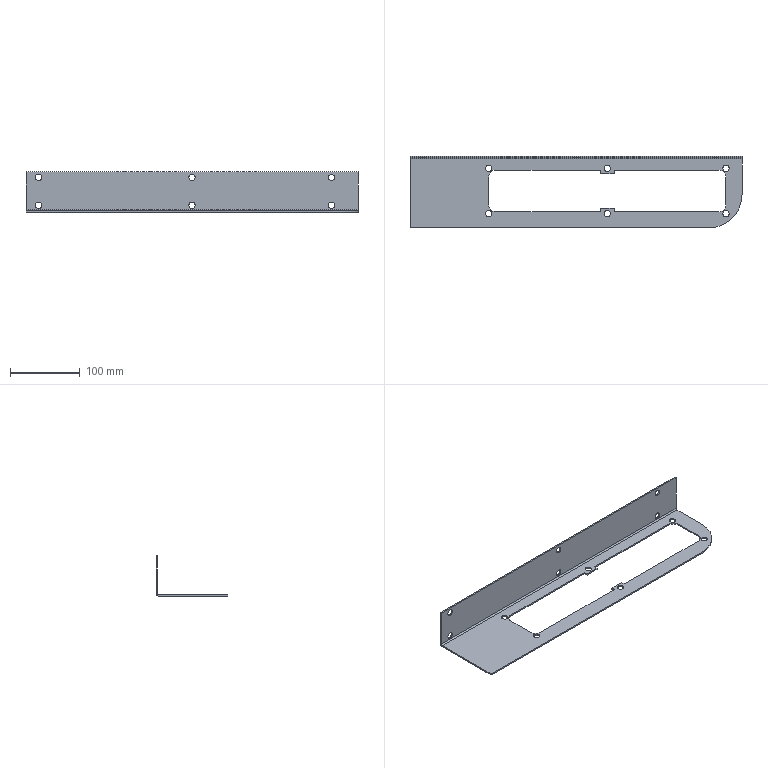Part | NX | features solid 2 | 1 solid | 51 faces | box 476 x 103 x 58 mm | volume 107387 mm3 | cylinder 31 | plane 20 | commonest cylinder face diameters 9 x20 9.2 x4 20 x4 4 x1 8 x1 96 x1